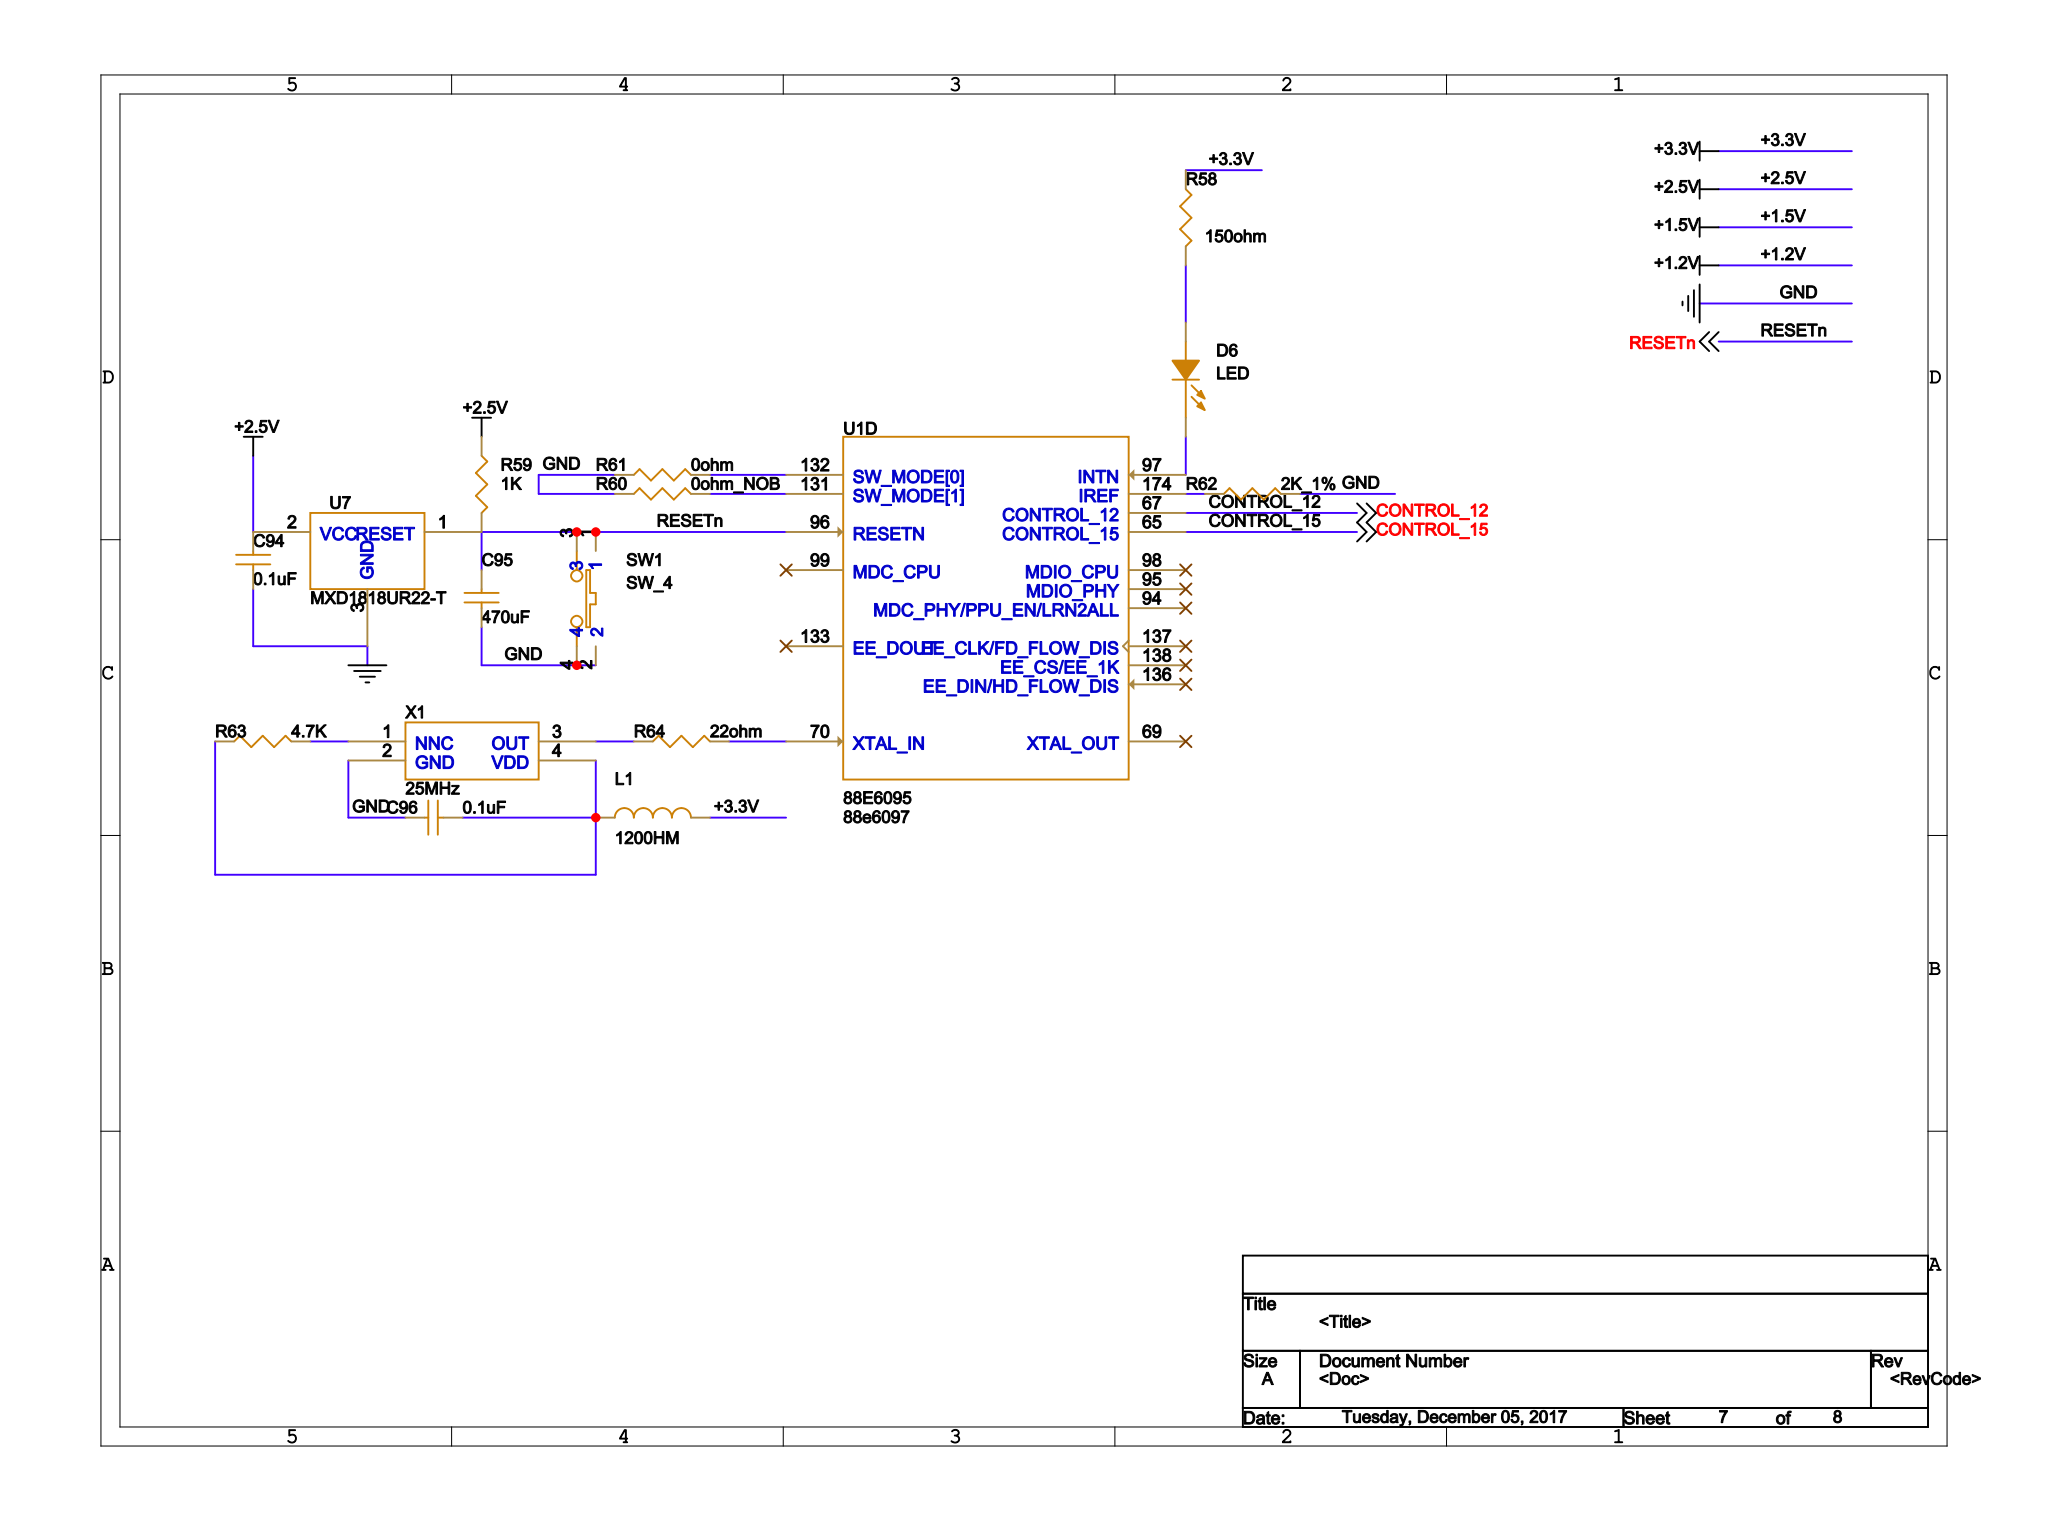Circuit board | Cadence Allegro | 219 parts | 174 nets | one sheet of the schematic
Parts on this sheet (reference | value | footprint):
C94 | 0.1uf | SC0603
C95 | 470uF | SC0603
C96 | 0.1uf | SC0603
D6 | LED | SD1206
L1 | 1200HM | SL0805
R58 | 150ohm | SR0603
R59 | 1K | SR0603
R60 | 0ohm_NOB | SR0603
R61 | 0ohm | SR0603
R62 | 2K_1% | SR0603
R63 | 4.7K | SR0603
R64 | 22ohm | SR0603
SW1 | SW_4 | SW-4
U1 | 88E6095 | 88E6097
U7 | MXD1818UR22-T | SOT23
X1 | 25MHz | SX4-0805A
Nets of these parts (net: part-pin ...):
GND: C94-2 C95-2 C96-1 R60-1 R61-1 R62-2 SW1-2 SW1-4 U7-3 X1-2
RESETN: C95-1 R59-2 SW1-1 SW1-3 U7-1 U1-96
CONTROL_12: U1-67
CONTROL_15: U1-65
N1346184: D6-2 U1-97
N1346262: R62-1 U1-174
N1345513: R61-2 U1-132
N1345566: R60-2 U1-131
N1346761: R64-2 U1-70
+2.5V: C94-1 R59-1 U7-2
+1.2V: U1-3 U1-8
+3.3V: L1-2 R58-1
N1346749: C96-2 L1-1 R63-1 X1-4
N1346188: D6-1 R58-2
N1346753: R63-2 X1-1
N1346757: R64-1 X1-3